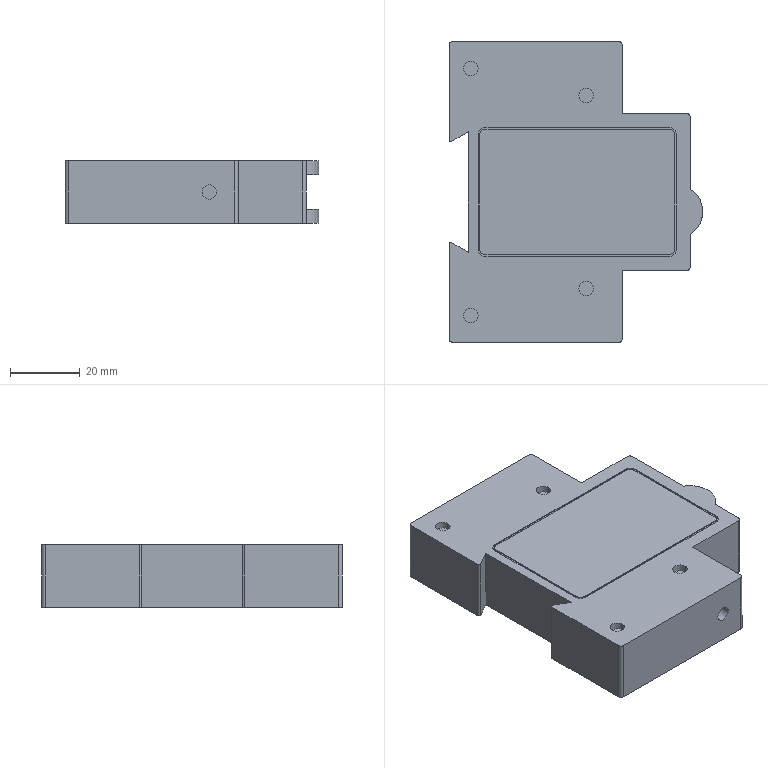Part | STEP file | 1 solid | 135 faces | box 72.568 x 86 x 18 mm | volume 87469 mm3 | plane 77 | cylinder 58 | commonest cylinder face diameters 4.125 x20 3 x8 4 x8 2 x6 15 x6 6.767 x4